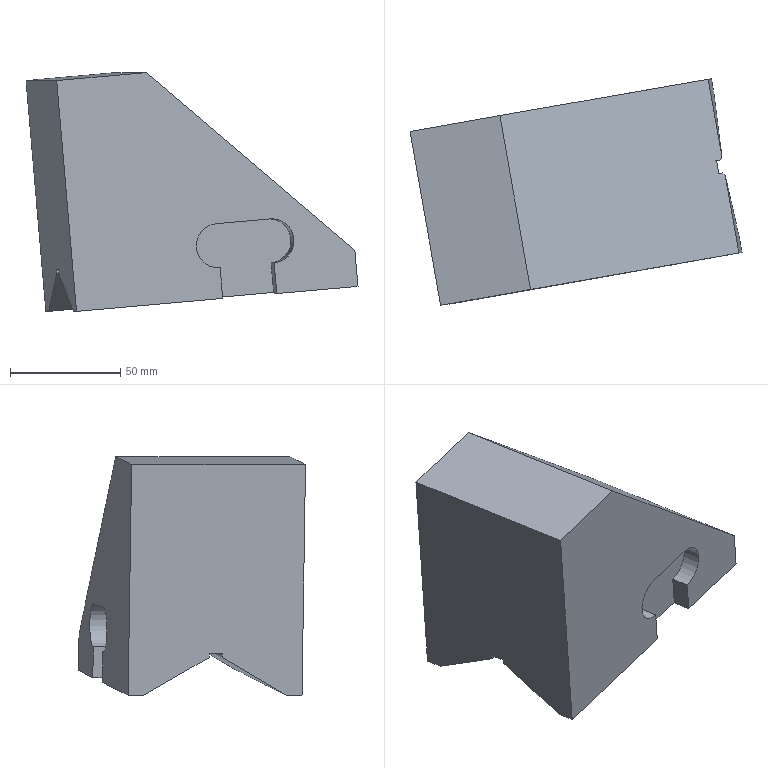Part | NX | features solid 2 | 1 solid | 28 faces | box 150.443 x 102.862 x 108.217 mm | volume 678258 mm3 | plane 24 | cylinder 4 | commonest cylinder face diameters 20 x4
STEP:
#1=CARTESIAN_POINT('',(1704.164,650.812,-11.2));
#2=VERTEX_POINT('',#1);
#3=CARTESIAN_POINT('',(1710.364,615.662,-11.208));
#4=VERTEX_POINT('',#3);
#5=CARTESIAN_POINT('',(1704.166,650.813,-11.208));
#6=DIRECTION('',(-0.1736,0.9848,0.));
#7=VECTOR('',#6,1000.);
#8=LINE('',#5,#7);
#9=EDGE_CURVE('',#2,#4,#8,.F.);
#10=ORIENTED_EDGE('',*,*,#9,.T.);
#11=CARTESIAN_POINT('',(1706.814,644.079,-27.658));
#12=VERTEX_POINT('',#11);
#13=CARTESIAN_POINT('',(1706.814,644.079,-27.658));
#14=DIRECTION('',(0.1075,-0.8604,0.4981));
#15=VECTOR('',#14,1000.);
#16=LINE('',#13,#15);
#17=EDGE_CURVE('',#12,#4,#16,.T.);
#18=ORIENTED_EDGE('',*,*,#17,.F.);
#19=CARTESIAN_POINT('',(1705.583,651.063,-27.658));
#20=VERTEX_POINT('',#19);
#21=CARTESIAN_POINT('',(1719.475,572.278,-27.658));
#22=DIRECTION('',(-0.1736,0.9848,0.));
#23=VECTOR('',#22,1000.);
#24=LINE('',#21,#23);
#25=EDGE_CURVE('',#12,#20,#24,.T.);
#26=ORIENTED_EDGE('',*,*,#25,.T.);
#27=CARTESIAN_POINT('',(1701.077,650.268,24.642));
#28=DIRECTION('',(-0.08583,-0.01513,0.9962));
#29=VECTOR('',#28,1000.);
#30=LINE('',#27,#29);
#31=EDGE_CURVE('',#20,#2,#30,.T.);
#32=ORIENTED_EDGE('',*,*,#31,.T.);
#33=EDGE_LOOP('',(#10,#18,#26,#32));
#34=FACE_BOUND('',#33,.T.);
#35=CARTESIAN_POINT('',(1714.969,571.483,24.642));
#36=DIRECTION('',(0.9811,0.173,0.08716));
#37=DIRECTION('',(-0.1736,0.9848,0.));
#38=AXIS2_PLACEMENT_3D('',#35,#36,#37);
#39=PLANE('',#38);
#40=ADVANCED_FACE('',(#34),#39,.T.);
#41=CARTESIAN_POINT('',(1709.785,614.233,-10.522));
#42=VERTEX_POINT('',#41);
#43=CARTESIAN_POINT('',(1582.987,591.875,-21.786));
#44=VERTEX_POINT('',#43);
#45=CARTESIAN_POINT('',(1710.526,614.363,-10.456));
#46=DIRECTION('',(-0.9811,-0.173,-0.08716));
#47=VECTOR('',#46,1000.);
#48=LINE('',#45,#47);
#49=EDGE_CURVE('',#42,#44,#48,.T.);
#50=ORIENTED_EDGE('',*,*,#49,.F.);
#51=CARTESIAN_POINT('',(1707.938,613.907,-8.947));
#52=VERTEX_POINT('',#51);
#53=CARTESIAN_POINT('',(1710.188,614.304,-10.865));
#54=DIRECTION('',(-0.7544,-0.133,0.6428));
#55=VECTOR('',#54,1000.);
#56=LINE('',#53,#55);
#57=EDGE_CURVE('',#42,#52,#56,.T.);
#58=ORIENTED_EDGE('',*,*,#57,.T.);
#59=CARTESIAN_POINT('',(1582.839,591.849,-20.061));
#60=VERTEX_POINT('',#59);
#61=CARTESIAN_POINT('',(1710.377,614.337,-8.731));
#62=DIRECTION('',(-0.9811,-0.173,-0.08716));
#63=VECTOR('',#62,1000.);
#64=LINE('',#61,#63);
#65=EDGE_CURVE('',#52,#60,#64,.T.);
#66=ORIENTED_EDGE('',*,*,#65,.T.);
#67=CARTESIAN_POINT('',(1575.457,590.547,65.61));
#68=DIRECTION('',(0.08583,0.01513,-0.9962));
#69=VECTOR('',#68,1000.);
#70=LINE('',#67,#69);
#71=EDGE_CURVE('',#44,#60,#70,.F.);
#72=ORIENTED_EDGE('',*,*,#71,.F.);
#73=EDGE_LOOP('',(#50,#58,#66,#72));
#74=FACE_BOUND('',#73,.T.);
#75=CARTESIAN_POINT('',(1710.526,614.363,-10.456));
#76=DIRECTION('',(0.1736,-0.9848,0.));
#77=DIRECTION('',(-0.08583,-0.01513,0.9962));
#78=AXIS2_PLACEMENT_3D('',#75,#76,#77);
#79=PLANE('',#78);
#80=ADVANCED_FACE('',(#74),#79,.T.);
#81=ORIENTED_EDGE('',*,*,#65,.F.);
#82=CARTESIAN_POINT('',(1708.979,607.998,-8.947));
#83=VERTEX_POINT('',#82);
#84=CARTESIAN_POINT('',(1707.938,613.907,-8.947));
#85=DIRECTION('',(0.1736,-0.9848,0.));
#86=VECTOR('',#85,1000.);
#87=LINE('',#84,#86);
#88=EDGE_CURVE('',#52,#83,#87,.T.);
#89=ORIENTED_EDGE('',*,*,#88,.T.);
#90=CARTESIAN_POINT('',(1583.881,585.94,-20.061));
#91=VERTEX_POINT('',#90);
#92=CARTESIAN_POINT('',(1711.419,608.428,-8.731));
#93=DIRECTION('',(-0.9811,-0.173,-0.08716));
#94=VECTOR('',#93,1000.);
#95=LINE('',#92,#94);
#96=EDGE_CURVE('',#83,#91,#95,.T.);
#97=ORIENTED_EDGE('',*,*,#96,.T.);
#98=CARTESIAN_POINT('',(1576.414,628.286,-20.061));
#99=DIRECTION('',(-0.1736,0.9848,0.));
#100=VECTOR('',#99,1000.);
#101=LINE('',#98,#100);
#102=EDGE_CURVE('',#60,#91,#101,.F.);
#103=ORIENTED_EDGE('',*,*,#102,.F.);
#104=EDGE_LOOP('',(#81,#89,#97,#103));
#105=FACE_BOUND('',#104,.T.);
#106=CARTESIAN_POINT('',(1710.377,614.337,-8.731));
#107=DIRECTION('',(0.08583,0.01513,-0.9962));
#108=DIRECTION('',(0.1736,-0.9848,0.));
#109=AXIS2_PLACEMENT_3D('',#106,#107,#108);
#110=PLANE('',#109);
#111=ADVANCED_FACE('',(#105),#110,.T.);
#112=ORIENTED_EDGE('',*,*,#96,.F.);
#113=CARTESIAN_POINT('',(1710.827,608.324,-10.522));
#114=VERTEX_POINT('',#113);
#115=CARTESIAN_POINT('',(1710.306,608.232,-10.078));
#116=DIRECTION('',(0.7544,0.133,-0.6428));
#117=VECTOR('',#116,1000.);
#118=LINE('',#115,#117);
#119=EDGE_CURVE('',#83,#114,#118,.T.);
#120=ORIENTED_EDGE('',*,*,#119,.T.);
#121=CARTESIAN_POINT('',(1584.029,585.966,-21.786));
#122=VERTEX_POINT('',#121);
#123=CARTESIAN_POINT('',(1711.568,608.454,-10.456));
#124=DIRECTION('',(-0.9811,-0.173,-0.08716));
#125=VECTOR('',#124,1000.);
#126=LINE('',#123,#125);
#127=EDGE_CURVE('',#114,#122,#126,.T.);
#128=ORIENTED_EDGE('',*,*,#127,.T.);
#129=CARTESIAN_POINT('',(1576.499,584.638,65.61));
#130=DIRECTION('',(-0.08583,-0.01513,0.9962));
#131=VECTOR('',#130,1000.);
#132=LINE('',#129,#131);
#133=EDGE_CURVE('',#91,#122,#132,.F.);
#134=ORIENTED_EDGE('',*,*,#133,.F.);
#135=EDGE_LOOP('',(#112,#120,#128,#134));
#136=FACE_BOUND('',#135,.T.);
#137=CARTESIAN_POINT('',(1711.419,608.428,-8.731));
#138=DIRECTION('',(-0.1736,0.9848,0.));
#139=DIRECTION('',(0.08583,0.01513,-0.9962));
#140=AXIS2_PLACEMENT_3D('',#137,#138,#139);
#141=PLANE('',#140);
#142=ADVANCED_FACE('',(#136),#141,.T.);
#143=CARTESIAN_POINT('',(1609.762,634.167,69.228));
#144=VERTEX_POINT('',#143);
#145=CARTESIAN_POINT('',(1623.653,555.382,69.228));
#146=VERTEX_POINT('',#145);
#147=CARTESIAN_POINT('',(1609.762,634.167,69.228));
#148=DIRECTION('',(0.1736,-0.9848,0.));
#149=VECTOR('',#148,1000.);
#150=LINE('',#147,#149);
#151=EDGE_CURVE('',#144,#146,#150,.T.);
#152=ORIENTED_EDGE('',*,*,#151,.F.);
#153=CARTESIAN_POINT('',(1569.032,626.985,65.61));
#154=VERTEX_POINT('',#153);
#155=CARTESIAN_POINT('',(1569.032,626.985,65.61));
#156=DIRECTION('',(0.9811,0.173,0.08716));
#157=VECTOR('',#156,1000.);
#158=LINE('',#155,#157);
#159=EDGE_CURVE('',#154,#144,#158,.T.);
#160=ORIENTED_EDGE('',*,*,#159,.F.);
#161=CARTESIAN_POINT('',(1582.924,548.2,65.61));
#162=VERTEX_POINT('',#161);
#163=CARTESIAN_POINT('',(1569.032,626.985,65.61));
#164=DIRECTION('',(0.1736,-0.9848,0.));
#165=VECTOR('',#164,1000.);
#166=LINE('',#163,#165);
#167=EDGE_CURVE('',#154,#162,#166,.T.);
#168=ORIENTED_EDGE('',*,*,#167,.T.);
#169=CARTESIAN_POINT('',(1582.924,548.2,65.61));
#170=DIRECTION('',(0.9811,0.173,0.08716));
#171=VECTOR('',#170,1000.);
#172=LINE('',#169,#171);
#173=EDGE_CURVE('',#162,#146,#172,.T.);
#174=ORIENTED_EDGE('',*,*,#173,.T.);
#175=EDGE_LOOP('',(#152,#160,#168,#174));
#176=FACE_BOUND('',#175,.T.);
#177=CARTESIAN_POINT('',(1569.032,626.985,65.61));
#178=DIRECTION('',(0.08583,0.01513,-0.9962));
#179=DIRECTION('',(0.9811,0.173,0.08716));
#180=AXIS2_PLACEMENT_3D('',#177,#178,#179);
#181=PLANE('',#180);
#182=ADVANCED_FACE('',(#176),#181,.F.);
#183=CARTESIAN_POINT('',(1711.86,607.178,-11.208));
#184=VERTEX_POINT('',#183);
#185=CARTESIAN_POINT('',(1718.244,579.261,-27.658));
#186=VERTEX_POINT('',#185);
#187=CARTESIAN_POINT('',(1711.568,608.454,-10.456));
#188=DIRECTION('',(0.1933,-0.8453,-0.4981));
#189=VECTOR('',#188,1000.);
#190=LINE('',#187,#189);
#191=EDGE_CURVE('',#184,#186,#190,.T.);
#192=ORIENTED_EDGE('',*,*,#191,.F.);
#193=CARTESIAN_POINT('',(1718.056,572.028,-11.2));
#194=VERTEX_POINT('',#193);
#195=CARTESIAN_POINT('',(1704.166,650.813,-11.208));
#196=DIRECTION('',(-0.1736,0.9848,0.));
#197=VECTOR('',#196,1000.);
#198=LINE('',#195,#197);
#199=EDGE_CURVE('',#184,#194,#198,.F.);
#200=ORIENTED_EDGE('',*,*,#199,.T.);
#201=CARTESIAN_POINT('',(1719.475,572.278,-27.658));
#202=VERTEX_POINT('',#201);
#203=CARTESIAN_POINT('',(1714.969,571.483,24.642));
#204=DIRECTION('',(0.08583,0.01513,-0.9962));
#205=VECTOR('',#204,1000.);
#206=LINE('',#203,#205);
#207=EDGE_CURVE('',#194,#202,#206,.T.);
#208=ORIENTED_EDGE('',*,*,#207,.T.);
#209=CARTESIAN_POINT('',(1719.475,572.278,-27.658));
#210=DIRECTION('',(-0.1736,0.9848,0.));
#211=VECTOR('',#210,1000.);
#212=LINE('',#209,#211);
#213=EDGE_CURVE('',#202,#186,#212,.T.);
#214=ORIENTED_EDGE('',*,*,#213,.T.);
#215=EDGE_LOOP('',(#192,#200,#208,#214));
#216=FACE_BOUND('',#215,.T.);
#217=CARTESIAN_POINT('',(1714.969,571.483,24.642));
#218=DIRECTION('',(0.9811,0.173,0.08716));
#219=DIRECTION('',(-0.1736,0.9848,0.));
#220=AXIS2_PLACEMENT_3D('',#217,#218,#219);
#221=PLANE('',#220);
#222=ADVANCED_FACE('',(#216),#221,.T.);
#223=CARTESIAN_POINT('',(1711.034,608.095,-10.659));
#224=DIRECTION('',(0.6116,-0.6787,-0.4065));
#225=VECTOR('',#224,1000.);
#226=LINE('',#223,#225);
#227=EDGE_CURVE('',#114,#184,#226,.T.);
#228=ORIENTED_EDGE('',*,*,#227,.T.);
#229=ORIENTED_EDGE('',*,*,#191,.T.);
#230=CARTESIAN_POINT('',(1681.454,572.774,-30.927));
#231=VERTEX_POINT('',#230);
#232=CARTESIAN_POINT('',(1718.244,579.261,-27.658));
#233=DIRECTION('',(-0.9811,-0.173,-0.08716));
#234=VECTOR('',#233,1000.);
#235=LINE('',#232,#234);
#236=EDGE_CURVE('',#186,#231,#235,.T.);
#237=ORIENTED_EDGE('',*,*,#236,.T.);
#238=CARTESIAN_POINT('',(1681.251,573.661,-30.404));
#239=VERTEX_POINT('',#238);
#240=CARTESIAN_POINT('',(1674.778,601.967,-13.725));
#241=DIRECTION('',(0.1933,-0.8453,-0.4981));
#242=VECTOR('',#241,1000.);
#243=LINE('',#240,#242);
#244=EDGE_CURVE('',#239,#231,#243,.T.);
#245=ORIENTED_EDGE('',*,*,#244,.F.);
#246=CARTESIAN_POINT('',(1656.725,569.337,-32.583));
#247=VERTEX_POINT('',#246);
#248=CARTESIAN_POINT('',(1718.041,580.148,-27.136));
#249=DIRECTION('',(-0.9811,-0.173,-0.08716));
#250=VECTOR('',#249,1000.);
#251=LINE('',#248,#250);
#252=EDGE_CURVE('',#239,#247,#251,.T.);
#253=ORIENTED_EDGE('',*,*,#252,.T.);
#254=CARTESIAN_POINT('',(1656.927,568.449,-33.106));
#255=VERTEX_POINT('',#254);
#256=CARTESIAN_POINT('',(1650.252,597.643,-15.903));
#257=DIRECTION('',(0.1933,-0.8453,-0.4981));
#258=VECTOR('',#257,1000.);
#259=LINE('',#256,#258);
#260=EDGE_CURVE('',#247,#255,#259,.T.);
#261=ORIENTED_EDGE('',*,*,#260,.T.);
#262=CARTESIAN_POINT('',(1590.705,556.773,-38.989));
#263=VERTEX_POINT('',#262);
#264=CARTESIAN_POINT('',(1718.244,579.261,-27.658));
#265=DIRECTION('',(-0.9811,-0.173,-0.08716));
#266=VECTOR('',#265,1000.);
#267=LINE('',#264,#266);
#268=EDGE_CURVE('',#255,#263,#267,.T.);
#269=ORIENTED_EDGE('',*,*,#268,.T.);
#270=CARTESIAN_POINT('',(1568.352,654.523,18.611));
#271=DIRECTION('',(-0.1933,0.8453,0.4981));
#272=VECTOR('',#271,1000.);
#273=LINE('',#270,#272);
#274=EDGE_CURVE('',#122,#263,#273,.F.);
#275=ORIENTED_EDGE('',*,*,#274,.F.);
#276=ORIENTED_EDGE('',*,*,#127,.F.);
#277=EDGE_LOOP('',(#228,#229,#237,#245,#253,#261,#269,#275,#276));
#278=FACE_BOUND('',#277,.T.);
#279=CARTESIAN_POINT('',(1711.568,608.454,-10.456));
#280=DIRECTION('',(-0.01249,0.5055,-0.8627));
#281=DIRECTION('',(0.1933,-0.8453,-0.4981));
#282=AXIS2_PLACEMENT_3D('',#279,#280,#281);
#283=PLANE('',#282);
#284=ADVANCED_FACE('',(#278),#283,.T.);
#285=ORIENTED_EDGE('',*,*,#17,.T.);
#286=CARTESIAN_POINT('',(1720.485,640.681,-23.217));
#287=DIRECTION('',(-0.3426,-0.847,0.4065));
#288=VECTOR('',#287,1000.);
#289=LINE('',#286,#288);
#290=EDGE_CURVE('',#4,#42,#289,.T.);
#291=ORIENTED_EDGE('',*,*,#290,.T.);
#292=ORIENTED_EDGE('',*,*,#49,.T.);
#293=CARTESIAN_POINT('',(1579.276,621.591,-38.989));
#294=VERTEX_POINT('',#293);
#295=CARTESIAN_POINT('',(1584.258,581.703,-15.898));
#296=DIRECTION('',(-0.1075,0.8604,-0.4981));
#297=VECTOR('',#296,1000.);
#298=LINE('',#295,#297);
#299=EDGE_CURVE('',#294,#44,#298,.F.);
#300=ORIENTED_EDGE('',*,*,#299,.F.);
#301=CARTESIAN_POINT('',(1645.498,633.267,-33.106));
#302=VERTEX_POINT('',#301);
#303=CARTESIAN_POINT('',(1706.814,644.079,-27.658));
#304=DIRECTION('',(-0.9811,-0.173,-0.08716));
#305=VECTOR('',#304,1000.);
#306=LINE('',#303,#305);
#307=EDGE_CURVE('',#302,#294,#306,.T.);
#308=ORIENTED_EDGE('',*,*,#307,.F.);
#309=CARTESIAN_POINT('',(1645.611,632.364,-32.583));
#310=VERTEX_POINT('',#309);
#311=CARTESIAN_POINT('',(1645.498,633.267,-33.106));
#312=DIRECTION('',(-0.1075,0.8604,-0.4981));
#313=VECTOR('',#312,1000.);
#314=LINE('',#311,#313);
#315=EDGE_CURVE('',#310,#302,#314,.T.);
#316=ORIENTED_EDGE('',*,*,#315,.F.);
#317=CARTESIAN_POINT('',(1670.138,636.689,-30.404));
#318=VERTEX_POINT('',#317);
#319=CARTESIAN_POINT('',(1706.927,643.176,-27.136));
#320=DIRECTION('',(0.9811,0.173,0.08716));
#321=VECTOR('',#320,1000.);
#322=LINE('',#319,#321);
#323=EDGE_CURVE('',#310,#318,#322,.T.);
#324=ORIENTED_EDGE('',*,*,#323,.T.);
#325=CARTESIAN_POINT('',(1670.025,637.592,-30.927));
#326=VERTEX_POINT('',#325);
#327=CARTESIAN_POINT('',(1670.025,637.592,-30.927));
#328=DIRECTION('',(-0.1075,0.8604,-0.4981));
#329=VECTOR('',#328,1000.);
#330=LINE('',#327,#329);
#331=EDGE_CURVE('',#318,#326,#330,.T.);
#332=ORIENTED_EDGE('',*,*,#331,.T.);
#333=CARTESIAN_POINT('',(1706.814,644.079,-27.658));
#334=DIRECTION('',(-0.9811,-0.173,-0.08716));
#335=VECTOR('',#334,1000.);
#336=LINE('',#333,#335);
#337=EDGE_CURVE('',#12,#326,#336,.T.);
#338=ORIENTED_EDGE('',*,*,#337,.F.);
#339=EDGE_LOOP('',(#285,#291,#292,#300,#308,#316,#324,#332,#338));
#340=FACE_BOUND('',#339,.T.);
#341=CARTESIAN_POINT('',(1706.814,644.079,-27.658));
#342=DIRECTION('',(0.1612,-0.4793,-0.8627));
#343=DIRECTION('',(0.1075,-0.8604,0.4981));
#344=AXIS2_PLACEMENT_3D('',#341,#342,#343);
#345=PLANE('',#344);
#346=ADVANCED_FACE('',(#340),#345,.T.);
#347=ORIENTED_EDGE('',*,*,#207,.F.);
#348=CARTESIAN_POINT('',(1718.048,572.026,-11.2));
#349=DIRECTION('',(-0.7544,-0.133,0.6428));
#350=VECTOR('',#349,1000.);
#351=LINE('',#348,#350);
#352=EDGE_CURVE('',#194,#146,#351,.T.);
#353=ORIENTED_EDGE('',*,*,#352,.T.);
#354=ORIENTED_EDGE('',*,*,#173,.F.);
#355=CARTESIAN_POINT('',(1591.936,549.789,-38.989));
#356=VERTEX_POINT('',#355);
#357=CARTESIAN_POINT('',(1582.924,548.2,65.61));
#358=DIRECTION('',(0.08583,0.01513,-0.9962));
#359=VECTOR('',#358,1000.);
#360=LINE('',#357,#359);
#361=EDGE_CURVE('',#356,#162,#360,.F.);
#362=ORIENTED_EDGE('',*,*,#361,.F.);
#363=CARTESIAN_POINT('',(1658.159,561.466,-33.106));
#364=VERTEX_POINT('',#363);
#365=CARTESIAN_POINT('',(1655.706,561.034,-33.324));
#366=DIRECTION('',(-0.9811,-0.173,-0.08716));
#367=VECTOR('',#366,1000.);
#368=LINE('',#365,#367);
#369=EDGE_CURVE('',#364,#356,#368,.T.);
#370=ORIENTED_EDGE('',*,*,#369,.F.);
#371=CARTESIAN_POINT('',(1656.957,561.254,-19.159));
#372=VERTEX_POINT('',#371);
#373=CARTESIAN_POINT('',(1659.532,561.708,-49.045));
#374=DIRECTION('',(-0.08583,-0.01513,0.9962));
#375=VECTOR('',#374,1000.);
#376=LINE('',#373,#375);
#377=EDGE_CURVE('',#364,#372,#376,.T.);
#378=ORIENTED_EDGE('',*,*,#377,.T.);
#379=CARTESIAN_POINT('',(1655.24,560.952,0.765));
#380=VERTEX_POINT('',#379);
#381=CARTESIAN_POINT('',(1656.099,561.103,-9.197));
#382=DIRECTION('',(-0.1736,0.9848,0.));
#383=DIRECTION('',(-0.9254,-0.1632,0.342));
#384=AXIS2_PLACEMENT_3D('',#381,#382,#383);
#385=CIRCLE('',#384,10.);
#386=EDGE_CURVE('',#372,#380,#385,.T.);
#387=ORIENTED_EDGE('',*,*,#386,.T.);
#388=CARTESIAN_POINT('',(1679.767,565.276,2.944));
#389=VERTEX_POINT('',#388);
#390=CARTESIAN_POINT('',(1655.24,560.952,0.765));
#391=DIRECTION('',(0.9811,0.173,0.08716));
#392=VECTOR('',#391,1000.);
#393=LINE('',#390,#392);
#394=EDGE_CURVE('',#380,#389,#393,.T.);
#395=ORIENTED_EDGE('',*,*,#394,.T.);
#396=CARTESIAN_POINT('',(1681.484,565.579,-16.98));
#397=VERTEX_POINT('',#396);
#398=CARTESIAN_POINT('',(1680.625,565.428,-7.018));
#399=DIRECTION('',(-0.1736,0.9848,0.));
#400=DIRECTION('',(-0.9254,-0.1632,0.342));
#401=AXIS2_PLACEMENT_3D('',#398,#399,#400);
#402=CIRCLE('',#401,10.);
#403=EDGE_CURVE('',#389,#397,#402,.T.);
#404=ORIENTED_EDGE('',*,*,#403,.T.);
#405=CARTESIAN_POINT('',(1682.685,565.791,-30.927));
#406=VERTEX_POINT('',#405);
#407=CARTESIAN_POINT('',(1681.484,565.579,-16.98));
#408=DIRECTION('',(-0.08583,-0.01513,0.9962));
#409=VECTOR('',#408,1000.);
#410=LINE('',#407,#409);
#411=EDGE_CURVE('',#406,#397,#410,.T.);
#412=ORIENTED_EDGE('',*,*,#411,.F.);
#413=CARTESIAN_POINT('',(1655.706,561.034,-33.324));
#414=DIRECTION('',(-0.9811,-0.173,-0.08716));
#415=VECTOR('',#414,1000.);
#416=LINE('',#413,#415);
#417=EDGE_CURVE('',#202,#406,#416,.T.);
#418=ORIENTED_EDGE('',*,*,#417,.F.);
#419=EDGE_LOOP('',(#347,#353,#354,#362,#370,#378,#387,#395,#404,#412,#418));
#420=FACE_BOUND('',#419,.T.);
#421=CARTESIAN_POINT('',(1651.2,560.239,18.977));
#422=DIRECTION('',(0.1736,-0.9848,0.));
#423=DIRECTION('',(0.9811,0.173,0.08716));
#424=AXIS2_PLACEMENT_3D('',#421,#422,#423);
#425=PLANE('',#424);
#426=ADVANCED_FACE('',(#420),#425,.T.);
#427=ORIENTED_EDGE('',*,*,#268,.F.);
#428=CARTESIAN_POINT('',(1658.159,561.466,-33.106));
#429=DIRECTION('',(0.1736,-0.9848,0.));
#430=VECTOR('',#429,1000.);
#431=LINE('',#428,#430);
#432=EDGE_CURVE('',#255,#364,#431,.T.);
#433=ORIENTED_EDGE('',*,*,#432,.T.);
#434=ORIENTED_EDGE('',*,*,#369,.T.);
#435=CARTESIAN_POINT('',(1591.936,549.789,-38.989));
#436=DIRECTION('',(0.1736,-0.9848,0.));
#437=VECTOR('',#436,1000.);
#438=LINE('',#435,#437);
#439=EDGE_CURVE('',#356,#263,#438,.F.);
#440=ORIENTED_EDGE('',*,*,#439,.T.);
#441=EDGE_LOOP('',(#427,#433,#434,#440));
#442=FACE_BOUND('',#441,.T.);
#443=CARTESIAN_POINT('',(1655.706,561.034,-33.324));
#444=DIRECTION('',(0.08583,0.01513,-0.9962));
#445=DIRECTION('',(0.1736,-0.9848,0.));
#446=AXIS2_PLACEMENT_3D('',#443,#444,#445);
#447=PLANE('',#446);
#448=ADVANCED_FACE('',(#442),#447,.T.);
#449=ORIENTED_EDGE('',*,*,#337,.T.);
#450=CARTESIAN_POINT('',(1668.793,644.575,-30.927));
#451=VERTEX_POINT('',#450);
#452=CARTESIAN_POINT('',(1682.685,565.791,-30.927));
#453=DIRECTION('',(-0.1736,0.9848,0.));
#454=VECTOR('',#453,1000.);
#455=LINE('',#452,#454);
#456=EDGE_CURVE('',#326,#451,#455,.T.);
#457=ORIENTED_EDGE('',*,*,#456,.T.);
#458=CARTESIAN_POINT('',(1641.814,639.818,-33.324));
#459=DIRECTION('',(0.9811,0.173,0.08716));
#460=VECTOR('',#459,1000.);
#461=LINE('',#458,#460);
#462=EDGE_CURVE('',#451,#20,#461,.T.);
#463=ORIENTED_EDGE('',*,*,#462,.T.);
#464=ORIENTED_EDGE('',*,*,#25,.F.);
#465=EDGE_LOOP('',(#449,#457,#463,#464));
#466=FACE_BOUND('',#465,.T.);
#467=CARTESIAN_POINT('',(1655.706,561.034,-33.324));
#468=DIRECTION('',(0.08583,0.01513,-0.9962));
#469=DIRECTION('',(0.1736,-0.9848,0.));
#470=AXIS2_PLACEMENT_3D('',#467,#468,#469);
#471=PLANE('',#470);
#472=ADVANCED_FACE('',(#466),#471,.T.);
#473=CARTESIAN_POINT('',(1682.685,565.791,-30.927));
#474=DIRECTION('',(0.1736,-0.9848,0.));
#475=VECTOR('',#474,1000.);
#476=LINE('',#473,#475);
#477=EDGE_CURVE('',#231,#406,#476,.T.);
#478=ORIENTED_EDGE('',*,*,#477,.F.);
#479=ORIENTED_EDGE('',*,*,#236,.F.);
#480=ORIENTED_EDGE('',*,*,#213,.F.);
#481=ORIENTED_EDGE('',*,*,#417,.T.);
#482=EDGE_LOOP('',(#478,#479,#480,#481));
#483=FACE_BOUND('',#482,.T.);
#484=CARTESIAN_POINT('',(1655.706,561.034,-33.324));
#485=DIRECTION('',(0.08583,0.01513,-0.9962));
#486=DIRECTION('',(0.1736,-0.9848,0.));
#487=AXIS2_PLACEMENT_3D('',#484,#485,#486);
#488=PLANE('',#487);
#489=ADVANCED_FACE('',(#483),#488,.T.);
#490=CARTESIAN_POINT('',(1644.267,640.251,-33.106));
#491=VERTEX_POINT('',#490);
#492=CARTESIAN_POINT('',(1658.159,561.466,-33.106));
#493=DIRECTION('',(-0.1736,0.9848,0.));
#494=VECTOR('',#493,1000.);
#495=LINE('',#492,#494);
#496=EDGE_CURVE('',#302,#491,#495,.T.);
#497=ORIENTED_EDGE('',*,*,#496,.F.);
#498=ORIENTED_EDGE('',*,*,#307,.T.);
#499=CARTESIAN_POINT('',(1578.045,628.574,-38.989));
#500=VERTEX_POINT('',#499);
#501=CARTESIAN_POINT('',(1591.936,549.789,-38.989));
#502=DIRECTION('',(0.1736,-0.9848,0.));
#503=VECTOR('',#502,1000.);
#504=LINE('',#501,#503);
#505=EDGE_CURVE('',#294,#500,#504,.F.);
#506=ORIENTED_EDGE('',*,*,#505,.T.);
#507=CARTESIAN_POINT('',(1641.814,639.818,-33.324));
#508=DIRECTION('',(0.9811,0.173,0.08716));
#509=VECTOR('',#508,1000.);
#510=LINE('',#507,#509);
#511=EDGE_CURVE('',#500,#491,#510,.T.);
#512=ORIENTED_EDGE('',*,*,#511,.T.);
#513=EDGE_LOOP('',(#497,#498,#506,#512));
#514=FACE_BOUND('',#513,.T.);
#515=CARTESIAN_POINT('',(1655.706,561.034,-33.324));
#516=DIRECTION('',(0.08583,0.01513,-0.9962));
#517=DIRECTION('',(0.1736,-0.9848,0.));
#518=AXIS2_PLACEMENT_3D('',#515,#516,#517);
#519=PLANE('',#518);
#520=ADVANCED_FACE('',(#514),#519,.T.);
#521=ORIENTED_EDGE('',*,*,#167,.F.);
#522=CARTESIAN_POINT('',(1573.538,627.779,13.311));
#523=DIRECTION('',(0.08583,0.01513,-0.9962));
#524=VECTOR('',#523,1000.);
#525=LINE('',#522,#524);
#526=EDGE_CURVE('',#154,#500,#525,.T.);
#527=ORIENTED_EDGE('',*,*,#526,.T.);
#528=ORIENTED_EDGE('',*,*,#505,.F.);
#529=ORIENTED_EDGE('',*,*,#299,.T.);
#530=ORIENTED_EDGE('',*,*,#71,.T.);
#531=ORIENTED_EDGE('',*,*,#102,.T.);
#532=ORIENTED_EDGE('',*,*,#133,.T.);
#533=ORIENTED_EDGE('',*,*,#274,.T.);
#534=ORIENTED_EDGE('',*,*,#439,.F.);
#535=ORIENTED_EDGE('',*,*,#361,.T.);
#536=EDGE_LOOP('',(#521,#527,#528,#529,#530,#531,#532,#533,#534,#535));
#537=FACE_BOUND('',#536,.T.);
#538=CARTESIAN_POINT('',(1569.032,626.985,65.61));
#539=DIRECTION('',(0.9811,0.173,0.08716));
#540=DIRECTION('',(0.1736,-0.9848,0.));
#541=AXIS2_PLACEMENT_3D('',#538,#539,#540);
#542=PLANE('',#541);
#543=ADVANCED_FACE('',(#537),#542,.F.);
#544=CARTESIAN_POINT('',(1704.156,650.811,-11.2));
#545=DIRECTION('',(-0.7544,-0.133,0.6428));
#546=VECTOR('',#545,1000.);
#547=LINE('',#544,#546);
#548=EDGE_CURVE('',#2,#144,#547,.T.);
#549=ORIENTED_EDGE('',*,*,#548,.F.);
#550=ORIENTED_EDGE('',*,*,#31,.F.);
#551=ORIENTED_EDGE('',*,*,#462,.F.);
#552=CARTESIAN_POINT('',(1667.592,644.364,-16.98));
#553=VERTEX_POINT('',#552);
#554=CARTESIAN_POINT('',(1670.167,644.818,-46.866));
#555=DIRECTION('',(-0.08583,-0.01513,0.9962));
#556=VECTOR('',#555,1000.);
#557=LINE('',#554,#556);
#558=EDGE_CURVE('',#451,#553,#557,.T.);
#559=ORIENTED_EDGE('',*,*,#558,.T.);
#560=CARTESIAN_POINT('',(1665.875,644.061,2.944));
#561=VERTEX_POINT('',#560);
#562=CARTESIAN_POINT('',(1666.733,644.212,-7.018));
#563=DIRECTION('',(-0.1736,0.9848,0.));
#564=DIRECTION('',(-0.9254,-0.1632,0.342));
#565=AXIS2_PLACEMENT_3D('',#562,#563,#564);
#566=CIRCLE('',#565,10.);
#567=EDGE_CURVE('',#561,#553,#566,.T.);
#568=ORIENTED_EDGE('',*,*,#567,.F.);
#569=CARTESIAN_POINT('',(1641.349,639.736,0.765));
#570=VERTEX_POINT('',#569);
#571=CARTESIAN_POINT('',(1665.875,644.061,2.944));
#572=DIRECTION('',(-0.9811,-0.173,-0.08716));
#573=VECTOR('',#572,1000.);
#574=LINE('',#571,#573);
#575=EDGE_CURVE('',#561,#570,#574,.T.);
#576=ORIENTED_EDGE('',*,*,#575,.T.);
#577=CARTESIAN_POINT('',(1643.065,640.039,-19.159));
#578=VERTEX_POINT('',#577);
#579=CARTESIAN_POINT('',(1642.207,639.888,-9.197));
#580=DIRECTION('',(-0.1736,0.9848,0.));
#581=DIRECTION('',(-0.9254,-0.1632,0.342));
#582=AXIS2_PLACEMENT_3D('',#579,#580,#581);
#583=CIRCLE('',#582,10.);
#584=EDGE_CURVE('',#578,#570,#583,.T.);
#585=ORIENTED_EDGE('',*,*,#584,.F.);
#586=CARTESIAN_POINT('',(1645.64,640.493,-49.045));
#587=DIRECTION('',(-0.08583,-0.01513,0.9962));
#588=VECTOR('',#587,1000.);
#589=LINE('',#586,#588);
#590=EDGE_CURVE('',#491,#578,#589,.T.);
#591=ORIENTED_EDGE('',*,*,#590,.F.);
#592=ORIENTED_EDGE('',*,*,#511,.F.);
#593=ORIENTED_EDGE('',*,*,#526,.F.);
#594=ORIENTED_EDGE('',*,*,#159,.T.);
#595=EDGE_LOOP('',(#549,#550,#551,#559,#568,#576,#585,#591,#592,#593,#594));
#596=FACE_BOUND('',#595,.T.);
#597=CARTESIAN_POINT('',(1637.308,639.024,18.977));
#598=DIRECTION('',(-0.1736,0.9848,0.));
#599=DIRECTION('',(-0.9811,-0.173,-0.08716));
#600=AXIS2_PLACEMENT_3D('',#597,#598,#599);
#601=PLANE('',#600);
#602=ADVANCED_FACE('',(#596),#601,.T.);
#603=ORIENTED_EDGE('',*,*,#584,.T.);
#604=CARTESIAN_POINT('',(1642.738,631.858,0.765));
#605=VERTEX_POINT('',#604);
#606=CARTESIAN_POINT('',(1642.738,631.858,0.765));
#607=DIRECTION('',(-0.1736,0.9848,0.));
#608=VECTOR('',#607,1000.);
#609=LINE('',#606,#608);
#610=EDGE_CURVE('',#605,#570,#609,.T.);
#611=ORIENTED_EDGE('',*,*,#610,.F.);
#612=CARTESIAN_POINT('',(1644.454,632.16,-19.159));
#613=VERTEX_POINT('',#612);
#614=CARTESIAN_POINT('',(1643.596,632.009,-9.197));
#615=DIRECTION('',(-0.1736,0.9848,0.));
#616=DIRECTION('',(-0.9254,-0.1632,0.342));
#617=AXIS2_PLACEMENT_3D('',#614,#615,#616);
#618=CIRCLE('',#617,10.);
#619=EDGE_CURVE('',#613,#605,#618,.T.);
#620=ORIENTED_EDGE('',*,*,#619,.F.);
#621=CARTESIAN_POINT('',(1644.454,632.16,-19.159));
#622=DIRECTION('',(-0.1736,0.9848,0.));
#623=VECTOR('',#622,1000.);
#624=LINE('',#621,#623);
#625=EDGE_CURVE('',#613,#578,#624,.T.);
#626=ORIENTED_EDGE('',*,*,#625,.T.);
#627=EDGE_LOOP('',(#603,#611,#620,#626));
#628=FACE_BOUND('',#627,.T.);
#629=CARTESIAN_POINT('',(1643.596,632.009,-9.197));
#630=DIRECTION('',(-0.1736,0.9848,0.));
#631=DIRECTION('',(-0.8925,-0.1574,0.4226));
#632=AXIS2_PLACEMENT_3D('',#629,#630,#631);
#633=CYLINDRICAL_SURFACE('',#632,10.);
#634=ADVANCED_FACE('',(#628),#633,.F.);
#635=ORIENTED_EDGE('',*,*,#575,.F.);
#636=CARTESIAN_POINT('',(1667.264,636.182,2.944));
#637=VERTEX_POINT('',#636);
#638=CARTESIAN_POINT('',(1667.264,636.182,2.944));
#639=DIRECTION('',(-0.1736,0.9848,0.));
#640=VECTOR('',#639,1000.);
#641=LINE('',#638,#640);
#642=EDGE_CURVE('',#637,#561,#641,.T.);
#643=ORIENTED_EDGE('',*,*,#642,.F.);
#644=CARTESIAN_POINT('',(1667.264,636.182,2.944));
#645=DIRECTION('',(-0.9811,-0.173,-0.08716));
#646=VECTOR('',#645,1000.);
#647=LINE('',#644,#646);
#648=EDGE_CURVE('',#637,#605,#647,.T.);
#649=ORIENTED_EDGE('',*,*,#648,.T.);
#650=ORIENTED_EDGE('',*,*,#610,.T.);
#651=EDGE_LOOP('',(#635,#643,#649,#650));
#652=FACE_BOUND('',#651,.T.);
#653=CARTESIAN_POINT('',(1667.264,636.182,2.944));
#654=DIRECTION('',(0.08583,0.01513,-0.9962));
#655=DIRECTION('',(-0.9811,-0.173,-0.08716));
#656=AXIS2_PLACEMENT_3D('',#653,#654,#655);
#657=PLANE('',#656);
#658=ADVANCED_FACE('',(#652),#657,.T.);
#659=ORIENTED_EDGE('',*,*,#567,.T.);
#660=CARTESIAN_POINT('',(1668.981,636.485,-16.98));
#661=VERTEX_POINT('',#660);
#662=CARTESIAN_POINT('',(1668.981,636.485,-16.98));
#663=DIRECTION('',(-0.1736,0.9848,0.));
#664=VECTOR('',#663,1000.);
#665=LINE('',#662,#664);
#666=EDGE_CURVE('',#661,#553,#665,.T.);
#667=ORIENTED_EDGE('',*,*,#666,.F.);
#668=CARTESIAN_POINT('',(1668.123,636.334,-7.018));
#669=DIRECTION('',(-0.1736,0.9848,0.));
#670=DIRECTION('',(-0.9254,-0.1632,0.342));
#671=AXIS2_PLACEMENT_3D('',#668,#669,#670);
#672=CIRCLE('',#671,10.);
#673=EDGE_CURVE('',#637,#661,#672,.T.);
#674=ORIENTED_EDGE('',*,*,#673,.F.);
#675=ORIENTED_EDGE('',*,*,#642,.T.);
#676=EDGE_LOOP('',(#659,#667,#674,#675));
#677=FACE_BOUND('',#676,.T.);
#678=CARTESIAN_POINT('',(1668.123,636.334,-7.018));
#679=DIRECTION('',(-0.1736,0.9848,0.));
#680=DIRECTION('',(-0.8925,-0.1574,0.4226));
#681=AXIS2_PLACEMENT_3D('',#678,#679,#680);
#682=CYLINDRICAL_SURFACE('',#681,10.);
#683=ADVANCED_FACE('',(#677),#682,.F.);
#684=ORIENTED_EDGE('',*,*,#673,.T.);
#685=CARTESIAN_POINT('',(1671.556,636.939,-46.866));
#686=DIRECTION('',(-0.08583,-0.01513,0.9962));
#687=VECTOR('',#686,1000.);
#688=LINE('',#685,#687);
#689=EDGE_CURVE('',#318,#661,#688,.T.);
#690=ORIENTED_EDGE('',*,*,#689,.F.);
#691=ORIENTED_EDGE('',*,*,#323,.F.);
#692=CARTESIAN_POINT('',(1647.029,632.614,-49.045));
#693=DIRECTION('',(-0.08583,-0.01513,0.9962));
#694=VECTOR('',#693,1000.);
#695=LINE('',#692,#694);
#696=EDGE_CURVE('',#310,#613,#695,.T.);
#697=ORIENTED_EDGE('',*,*,#696,.T.);
#698=ORIENTED_EDGE('',*,*,#619,.T.);
#699=ORIENTED_EDGE('',*,*,#648,.F.);
#700=EDGE_LOOP('',(#684,#690,#691,#697,#698,#699));
#701=FACE_BOUND('',#700,.T.);
#702=CARTESIAN_POINT('',(1643.596,632.009,-9.197));
#703=DIRECTION('',(-0.1736,0.9848,0.));
#704=DIRECTION('',(-0.8925,-0.1574,0.4226));
#705=AXIS2_PLACEMENT_3D('',#702,#703,#704);
#706=PLANE('',#705);
#707=ADVANCED_FACE('',(#701),#706,.T.);
#708=ORIENTED_EDGE('',*,*,#496,.T.);
#709=ORIENTED_EDGE('',*,*,#590,.T.);
#710=ORIENTED_EDGE('',*,*,#625,.F.);
#711=ORIENTED_EDGE('',*,*,#696,.F.);
#712=ORIENTED_EDGE('',*,*,#315,.T.);
#713=EDGE_LOOP('',(#708,#709,#710,#711,#712));
#714=FACE_BOUND('',#713,.T.);
#715=CARTESIAN_POINT('',(1647.029,632.614,-49.045));
#716=DIRECTION('',(-0.9811,-0.173,-0.08716));
#717=DIRECTION('',(-0.08583,-0.01513,0.9962));
#718=AXIS2_PLACEMENT_3D('',#715,#716,#717);
#719=PLANE('',#718);
#720=ADVANCED_FACE('',(#714),#719,.F.);
#721=ORIENTED_EDGE('',*,*,#331,.F.);
#722=ORIENTED_EDGE('',*,*,#689,.T.);
#723=ORIENTED_EDGE('',*,*,#666,.T.);
#724=ORIENTED_EDGE('',*,*,#558,.F.);
#725=ORIENTED_EDGE('',*,*,#456,.F.);
#726=EDGE_LOOP('',(#721,#722,#723,#724,#725));
#727=FACE_BOUND('',#726,.T.);
#728=CARTESIAN_POINT('',(1671.556,636.939,-46.866));
#729=DIRECTION('',(-0.9811,-0.173,-0.08716));
#730=DIRECTION('',(-0.08583,-0.01513,0.9962));
#731=AXIS2_PLACEMENT_3D('',#728,#729,#730);
#732=PLANE('',#731);
#733=ADVANCED_FACE('',(#727),#732,.T.);
#734=ORIENTED_EDGE('',*,*,#394,.F.);
#735=CARTESIAN_POINT('',(1653.851,568.83,0.765));
#736=VERTEX_POINT('',#735);
#737=CARTESIAN_POINT('',(1653.851,568.83,0.765));
#738=DIRECTION('',(0.1736,-0.9848,0.));
#739=VECTOR('',#738,1000.);
#740=LINE('',#737,#739);
#741=EDGE_CURVE('',#736,#380,#740,.T.);
#742=ORIENTED_EDGE('',*,*,#741,.F.);
#743=CARTESIAN_POINT('',(1678.378,573.155,2.944));
#744=VERTEX_POINT('',#743);
#745=CARTESIAN_POINT('',(1653.851,568.83,0.765));
#746=DIRECTION('',(0.9811,0.173,0.08716));
#747=VECTOR('',#746,1000.);
#748=LINE('',#745,#747);
#749=EDGE_CURVE('',#736,#744,#748,.T.);
#750=ORIENTED_EDGE('',*,*,#749,.T.);
#751=CARTESIAN_POINT('',(1679.767,565.276,2.944));
#752=DIRECTION('',(-0.1736,0.9848,0.));
#753=VECTOR('',#752,1000.);
#754=LINE('',#751,#753);
#755=EDGE_CURVE('',#389,#744,#754,.T.);
#756=ORIENTED_EDGE('',*,*,#755,.F.);
#757=EDGE_LOOP('',(#734,#742,#750,#756));
#758=FACE_BOUND('',#757,.T.);
#759=CARTESIAN_POINT('',(1653.851,568.83,0.765));
#760=DIRECTION('',(0.08583,0.01513,-0.9962));
#761=DIRECTION('',(-0.9811,-0.173,-0.08716));
#762=AXIS2_PLACEMENT_3D('',#759,#760,#761);
#763=PLANE('',#762);
#764=ADVANCED_FACE('',(#758),#763,.T.);
#765=CARTESIAN_POINT('',(1655.568,569.133,-19.159));
#766=VERTEX_POINT('',#765);
#767=CARTESIAN_POINT('',(1656.957,561.254,-19.159));
#768=DIRECTION('',(-0.1736,0.9848,0.));
#769=VECTOR('',#768,1000.);
#770=LINE('',#767,#769);
#771=EDGE_CURVE('',#372,#766,#770,.T.);
#772=ORIENTED_EDGE('',*,*,#771,.F.);
#773=ORIENTED_EDGE('',*,*,#377,.F.);
#774=ORIENTED_EDGE('',*,*,#432,.F.);
#775=ORIENTED_EDGE('',*,*,#260,.F.);
#776=CARTESIAN_POINT('',(1658.143,569.587,-49.045));
#777=DIRECTION('',(-0.08583,-0.01513,0.9962));
#778=VECTOR('',#777,1000.);
#779=LINE('',#776,#778);
#780=EDGE_CURVE('',#247,#766,#779,.T.);
#781=ORIENTED_EDGE('',*,*,#780,.T.);
#782=EDGE_LOOP('',(#772,#773,#774,#775,#781));
#783=FACE_BOUND('',#782,.T.);
#784=CARTESIAN_POINT('',(1658.143,569.587,-49.045));
#785=DIRECTION('',(0.9811,0.173,0.08716));
#786=DIRECTION('',(0.08583,0.01513,-0.9962));
#787=AXIS2_PLACEMENT_3D('',#784,#785,#786);
#788=PLANE('',#787);
#789=ADVANCED_FACE('',(#783),#788,.T.);
#790=ORIENTED_EDGE('',*,*,#411,.T.);
#791=CARTESIAN_POINT('',(1680.094,573.457,-16.98));
#792=VERTEX_POINT('',#791);
#793=CARTESIAN_POINT('',(1681.484,565.579,-16.98));
#794=DIRECTION('',(-0.1736,0.9848,0.));
#795=VECTOR('',#794,1000.);
#796=LINE('',#793,#795);
#797=EDGE_CURVE('',#397,#792,#796,.T.);
#798=ORIENTED_EDGE('',*,*,#797,.T.);
#799=CARTESIAN_POINT('',(1680.094,573.457,-16.98));
#800=DIRECTION('',(-0.08583,-0.01513,0.9962));
#801=VECTOR('',#800,1000.);
#802=LINE('',#799,#801);
#803=EDGE_CURVE('',#239,#792,#802,.T.);
#804=ORIENTED_EDGE('',*,*,#803,.F.);
#805=ORIENTED_EDGE('',*,*,#244,.T.);
#806=ORIENTED_EDGE('',*,*,#477,.T.);
#807=EDGE_LOOP('',(#790,#798,#804,#805,#806));
#808=FACE_BOUND('',#807,.T.);
#809=CARTESIAN_POINT('',(1680.094,573.457,-16.98));
#810=DIRECTION('',(0.9811,0.173,0.08716));
#811=DIRECTION('',(0.08583,0.01513,-0.9962));
#812=AXIS2_PLACEMENT_3D('',#809,#810,#811);
#813=PLANE('',#812);
#814=ADVANCED_FACE('',(#808),#813,.F.);
#815=CARTESIAN_POINT('',(1679.236,573.306,-7.018));
#816=DIRECTION('',(-0.1736,0.9848,0.));
#817=DIRECTION('',(-0.9254,-0.1632,0.342));
#818=AXIS2_PLACEMENT_3D('',#815,#816,#817);
#819=CIRCLE('',#818,10.);
#820=EDGE_CURVE('',#744,#792,#819,.T.);
#821=ORIENTED_EDGE('',*,*,#820,.F.);
#822=ORIENTED_EDGE('',*,*,#749,.F.);
#823=CARTESIAN_POINT('',(1654.71,568.981,-9.197));
#824=DIRECTION('',(-0.1736,0.9848,0.));
#825=DIRECTION('',(-0.9254,-0.1632,0.342));
#826=AXIS2_PLACEMENT_3D('',#823,#824,#825);
#827=CIRCLE('',#826,10.);
#828=EDGE_CURVE('',#766,#736,#827,.T.);
#829=ORIENTED_EDGE('',*,*,#828,.F.);
#830=ORIENTED_EDGE('',*,*,#780,.F.);
#831=ORIENTED_EDGE('',*,*,#252,.F.);
#832=ORIENTED_EDGE('',*,*,#803,.T.);
#833=EDGE_LOOP('',(#821,#822,#829,#830,#831,#832));
#834=FACE_BOUND('',#833,.T.);
#835=CARTESIAN_POINT('',(1652.135,568.527,20.689));
#836=DIRECTION('',(0.1736,-0.9848,0.));
#837=DIRECTION('',(-0.8925,-0.1574,0.4226));
#838=AXIS2_PLACEMENT_3D('',#835,#836,#837);
#839=PLANE('',#838);
#840=ADVANCED_FACE('',(#834),#839,.T.);
#841=ORIENTED_EDGE('',*,*,#820,.T.);
#842=ORIENTED_EDGE('',*,*,#797,.F.);
#843=ORIENTED_EDGE('',*,*,#403,.F.);
#844=ORIENTED_EDGE('',*,*,#755,.T.);
#845=EDGE_LOOP('',(#841,#842,#843,#844));
#846=FACE_BOUND('',#845,.T.);
#847=CARTESIAN_POINT('',(1680.625,565.428,-7.018));
#848=DIRECTION('',(-0.1736,0.9848,0.));
#849=DIRECTION('',(-0.8925,-0.1574,0.4226));
#850=AXIS2_PLACEMENT_3D('',#847,#848,#849);
#851=CYLINDRICAL_SURFACE('',#850,10.);
#852=ADVANCED_FACE('',(#846),#851,.F.);
#853=ORIENTED_EDGE('',*,*,#828,.T.);
#854=ORIENTED_EDGE('',*,*,#741,.T.);
#855=ORIENTED_EDGE('',*,*,#386,.F.);
#856=ORIENTED_EDGE('',*,*,#771,.T.);
#857=EDGE_LOOP('',(#853,#854,#855,#856));
#858=FACE_BOUND('',#857,.T.);
#859=CARTESIAN_POINT('',(1656.099,561.103,-9.197));
#860=DIRECTION('',(-0.1736,0.9848,0.));
#861=DIRECTION('',(-0.8925,-0.1574,0.4226));
#862=AXIS2_PLACEMENT_3D('',#859,#860,#861);
#863=CYLINDRICAL_SURFACE('',#862,10.);
#864=ADVANCED_FACE('',(#858),#863,.F.);
#865=ORIENTED_EDGE('',*,*,#119,.F.);
#866=ORIENTED_EDGE('',*,*,#88,.F.);
#867=ORIENTED_EDGE('',*,*,#57,.F.);
#868=ORIENTED_EDGE('',*,*,#290,.F.);
#869=ORIENTED_EDGE('',*,*,#9,.F.);
#870=ORIENTED_EDGE('',*,*,#548,.T.);
#871=ORIENTED_EDGE('',*,*,#151,.T.);
#872=ORIENTED_EDGE('',*,*,#352,.F.);
#873=ORIENTED_EDGE('',*,*,#199,.F.);
#874=ORIENTED_EDGE('',*,*,#227,.F.);
#875=EDGE_LOOP('',(#865,#866,#867,#868,#869,#870,#871,#872,#873,#874));
#876=FACE_BOUND('',#875,.T.);
#877=CARTESIAN_POINT('',(1704.156,650.811,-11.2));
#878=DIRECTION('',(0.633,0.1116,0.766));
#879=DIRECTION('',(-0.7544,-0.133,0.6428));
#880=AXIS2_PLACEMENT_3D('',#877,#878,#879);
#881=PLANE('',#880);
#882=ADVANCED_FACE('',(#876),#881,.T.);
#883=CLOSED_SHELL('',(#40,#80,#111,#142,#182,#222,#284,#346,#426,#448,#472,#489,#520,#543,#602,#634,#658,#683,#707,#720,#733,#764,#789,#814,#840,#852,#864,#882));
#884=MANIFOLD_SOLID_BREP('',#883);
#885=(LENGTH_UNIT()NAMED_UNIT(*)SI_UNIT(.MILLI.,.METRE.));
#886=UNCERTAINTY_MEASURE_WITH_UNIT(LENGTH_MEASURE(0.02045),#885,'','');
#887=(NAMED_UNIT(*)PLANE_ANGLE_UNIT()SI_UNIT($,.RADIAN.));
#888=(NAMED_UNIT(*)SI_UNIT($,.STERADIAN.)SOLID_ANGLE_UNIT());
#889=(GEOMETRIC_REPRESENTATION_CONTEXT(3)GLOBAL_UNCERTAINTY_ASSIGNED_CONTEXT((#886))GLOBAL_UNIT_ASSIGNED_CONTEXT((#885,#887,#888))REPRESENTATION_CONTEXT('',''));
#890=ADVANCED_BREP_SHAPE_REPRESENTATION('',(#884),#889);